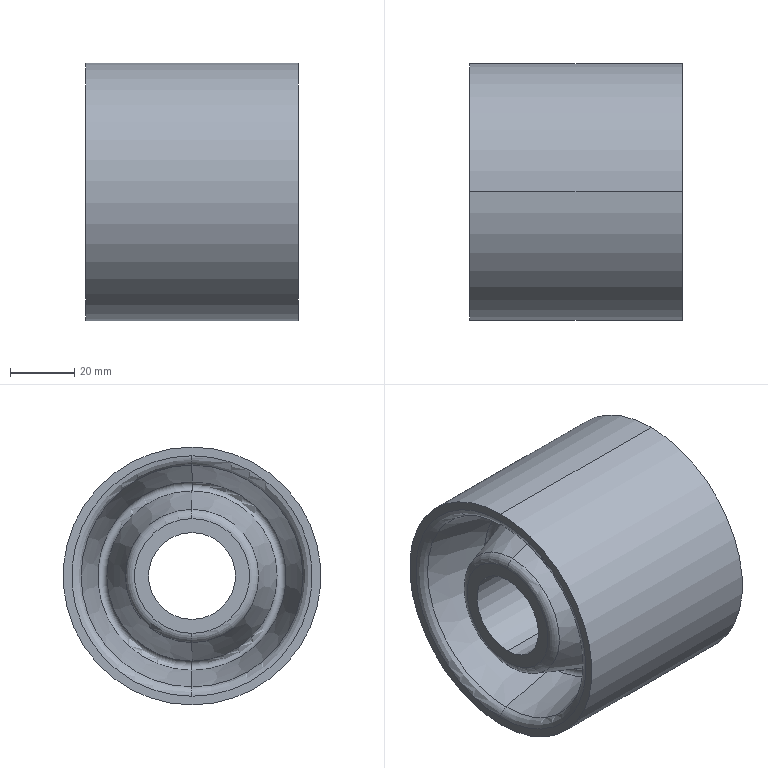Part | SolidWorks | features Revolution 1 | 1 solid | 28 faces | box 66 x 80 x 80 mm | volume 217017 mm3 | torus 12 | cone 8 | cylinder 4 | plane 4 | commonest cylinder face diameters 27 x2 80 x2
STEP:
#1=CARTESIAN_POINT('',(0.,0.,37.321));
#2=VERTEX_POINT('',#1);
#3=CARTESIAN_POINT('',(0.,0.,-37.321));
#4=VERTEX_POINT('',#3);
#5=CARTESIAN_POINT('',(0.,0.,0.));
#6=DIRECTION('',(-1.,0.,0.));
#7=DIRECTION('',(0.,0.,1.));
#8=AXIS2_PLACEMENT_3D('',#5,#6,#7);
#9=CIRCLE('',#8,37.321);
#10=EDGE_CURVE('',#2,#4,#9,.T.);
#11=ORIENTED_EDGE('',*,*,#10,.T.);
#12=CARTESIAN_POINT('',(2.247,0.,-34.417));
#13=VERTEX_POINT('',#12);
#14=CARTESIAN_POINT('',(3.,0.,-37.321));
#15=DIRECTION('',(0.,1.,0.));
#16=DIRECTION('',(0.,0.,1.));
#17=AXIS2_PLACEMENT_3D('',#14,#15,#16);
#18=CIRCLE('',#17,3.);
#19=EDGE_CURVE('',#4,#13,#18,.T.);
#20=ORIENTED_EDGE('',*,*,#19,.T.);
#21=CARTESIAN_POINT('',(2.247,0.,34.417));
#22=VERTEX_POINT('',#21);
#23=CARTESIAN_POINT('',(2.247,0.,0.));
#24=DIRECTION('',(-1.,0.,0.));
#25=DIRECTION('',(0.,0.,1.));
#26=AXIS2_PLACEMENT_3D('',#23,#24,#25);
#27=CIRCLE('',#26,34.417);
#28=EDGE_CURVE('',#22,#13,#27,.T.);
#29=ORIENTED_EDGE('',*,*,#28,.F.);
#30=CARTESIAN_POINT('',(3.,0.,37.321));
#31=DIRECTION('',(0.,-1.,0.));
#32=DIRECTION('',(0.,0.,-1.));
#33=AXIS2_PLACEMENT_3D('',#30,#31,#32);
#34=CIRCLE('',#33,3.);
#35=EDGE_CURVE('',#2,#22,#34,.T.);
#36=ORIENTED_EDGE('',*,*,#35,.F.);
#37=EDGE_LOOP('',(#11,#20,#29,#36));
#38=FACE_OUTER_BOUND('',#37,.T.);
#39=CARTESIAN_POINT('',(3.,0.,0.));
#40=DIRECTION('',(-1.,0.,0.));
#41=DIRECTION('',(0.,0.,1.));
#42=AXIS2_PLACEMENT_3D('',#39,#40,#41);
#43=TOROIDAL_SURFACE('',#42,37.321,3.);
#44=ADVANCED_FACE('',(#38),#43,.T.);
#45=CARTESIAN_POINT('',(22.093,0.,-29.272));
#46=VERTEX_POINT('',#45);
#47=CARTESIAN_POINT('',(22.093,0.,29.272));
#48=VERTEX_POINT('',#47);
#49=CARTESIAN_POINT('',(22.093,0.,0.));
#50=DIRECTION('',(-1.,0.,0.));
#51=DIRECTION('',(0.,0.,1.));
#52=AXIS2_PLACEMENT_3D('',#49,#50,#51);
#53=CIRCLE('',#52,29.272);
#54=EDGE_CURVE('',#46,#48,#53,.T.);
#55=ORIENTED_EDGE('',*,*,#54,.F.);
#56=CARTESIAN_POINT('',(2.247,0.,-34.417));
#57=DIRECTION('',(-0.968,0.,-0.251));
#58=VECTOR('',#57,1000.);
#59=LINE('',#56,#58);
#60=EDGE_CURVE('',#46,#13,#59,.T.);
#61=ORIENTED_EDGE('',*,*,#60,.T.);
#62=CARTESIAN_POINT('',(2.247,0.,0.));
#63=DIRECTION('',(-1.,0.,0.));
#64=DIRECTION('',(0.,0.,1.));
#65=AXIS2_PLACEMENT_3D('',#62,#63,#64);
#66=CIRCLE('',#65,34.417);
#67=EDGE_CURVE('',#13,#22,#66,.T.);
#68=ORIENTED_EDGE('',*,*,#67,.T.);
#69=CARTESIAN_POINT('',(2.247,0.,34.417));
#70=DIRECTION('',(-0.968,0.,0.251));
#71=VECTOR('',#70,1000.);
#72=LINE('',#69,#71);
#73=EDGE_CURVE('',#48,#22,#72,.T.);
#74=ORIENTED_EDGE('',*,*,#73,.F.);
#75=EDGE_LOOP('',(#55,#61,#68,#74));
#76=FACE_OUTER_BOUND('',#75,.T.);
#77=CARTESIAN_POINT('',(2.247,0.,0.));
#78=DIRECTION('',(-1.,0.,0.));
#79=DIRECTION('',(0.,0.,1.));
#80=AXIS2_PLACEMENT_3D('',#77,#78,#79);
#81=CONICAL_SURFACE('',#80,34.417,0.2537);
#82=ADVANCED_FACE('',(#76),#81,.F.);
#83=CARTESIAN_POINT('',(22.191,0.,-26.397));
#84=VERTEX_POINT('',#83);
#85=CARTESIAN_POINT('',(22.191,0.,26.397));
#86=VERTEX_POINT('',#85);
#87=CARTESIAN_POINT('',(22.191,0.,0.));
#88=DIRECTION('',(-1.,0.,0.));
#89=DIRECTION('',(0.,0.,1.));
#90=AXIS2_PLACEMENT_3D('',#87,#88,#89);
#91=CIRCLE('',#90,26.397);
#92=EDGE_CURVE('',#84,#86,#91,.T.);
#93=ORIENTED_EDGE('',*,*,#92,.F.);
#94=CARTESIAN_POINT('',(21.717,0.,-27.82));
#95=DIRECTION('',(0.,1.,0.));
#96=DIRECTION('',(0.,0.,1.));
#97=AXIS2_PLACEMENT_3D('',#94,#95,#96);
#98=CIRCLE('',#97,1.5);
#99=EDGE_CURVE('',#84,#46,#98,.T.);
#100=ORIENTED_EDGE('',*,*,#99,.T.);
#101=ORIENTED_EDGE('',*,*,#54,.T.);
#102=CARTESIAN_POINT('',(21.717,0.,27.82));
#103=DIRECTION('',(0.,-1.,0.));
#104=DIRECTION('',(0.,0.,-1.));
#105=AXIS2_PLACEMENT_3D('',#102,#103,#104);
#106=CIRCLE('',#105,1.5);
#107=EDGE_CURVE('',#86,#48,#106,.T.);
#108=ORIENTED_EDGE('',*,*,#107,.F.);
#109=EDGE_LOOP('',(#93,#100,#101,#108));
#110=FACE_OUTER_BOUND('',#109,.T.);
#111=CARTESIAN_POINT('',(21.717,0.,0.));
#112=DIRECTION('',(-1.,0.,0.));
#113=DIRECTION('',(0.,0.,1.));
#114=AXIS2_PLACEMENT_3D('',#111,#112,#113);
#115=TOROIDAL_SURFACE('',#114,27.82,1.5);
#116=ADVANCED_FACE('',(#110),#115,.F.);
#117=CARTESIAN_POINT('',(5.051,0.,20.684));
#118=VERTEX_POINT('',#117);
#119=CARTESIAN_POINT('',(5.051,0.,-20.684));
#120=VERTEX_POINT('',#119);
#121=CARTESIAN_POINT('',(5.051,0.,0.));
#122=DIRECTION('',(-1.,0.,0.));
#123=DIRECTION('',(0.,0.,1.));
#124=AXIS2_PLACEMENT_3D('',#121,#122,#123);
#125=CIRCLE('',#124,20.684);
#126=EDGE_CURVE('',#118,#120,#125,.T.);
#127=ORIENTED_EDGE('',*,*,#126,.F.);
#128=CARTESIAN_POINT('',(22.191,0.,26.397));
#129=DIRECTION('',(0.9487,0.,0.3162));
#130=VECTOR('',#129,1000.);
#131=LINE('',#128,#130);
#132=EDGE_CURVE('',#118,#86,#131,.T.);
#133=ORIENTED_EDGE('',*,*,#132,.T.);
#134=CARTESIAN_POINT('',(22.191,0.,0.));
#135=DIRECTION('',(-1.,0.,0.));
#136=DIRECTION('',(0.,0.,1.));
#137=AXIS2_PLACEMENT_3D('',#134,#135,#136);
#138=CIRCLE('',#137,26.397);
#139=EDGE_CURVE('',#86,#84,#138,.T.);
#140=ORIENTED_EDGE('',*,*,#139,.T.);
#141=CARTESIAN_POINT('',(22.191,0.,-26.397));
#142=DIRECTION('',(0.9487,0.,-0.3162));
#143=VECTOR('',#142,1000.);
#144=LINE('',#141,#143);
#145=EDGE_CURVE('',#120,#84,#144,.T.);
#146=ORIENTED_EDGE('',*,*,#145,.F.);
#147=EDGE_LOOP('',(#127,#133,#140,#146));
#148=FACE_OUTER_BOUND('',#147,.T.);
#149=CARTESIAN_POINT('',(22.191,0.,0.));
#150=DIRECTION('',(1.,0.,0.));
#151=DIRECTION('',(0.,0.,-1.));
#152=AXIS2_PLACEMENT_3D('',#149,#150,#151);
#153=CONICAL_SURFACE('',#152,26.397,0.3218);
#154=ADVANCED_FACE('',(#148),#153,.T.);
#155=ORIENTED_EDGE('',*,*,#126,.T.);
#156=CARTESIAN_POINT('',(3.,0.,-17.838));
#157=VERTEX_POINT('',#156);
#158=CARTESIAN_POINT('',(6.,0.,-17.838));
#159=DIRECTION('',(0.,1.,0.));
#160=DIRECTION('',(0.,0.,1.));
#161=AXIS2_PLACEMENT_3D('',#158,#159,#160);
#162=CIRCLE('',#161,3.);
#163=EDGE_CURVE('',#120,#157,#162,.T.);
#164=ORIENTED_EDGE('',*,*,#163,.T.);
#165=CARTESIAN_POINT('',(3.,0.,17.838));
#166=VERTEX_POINT('',#165);
#167=CARTESIAN_POINT('',(3.,0.,0.));
#168=DIRECTION('',(-1.,0.,0.));
#169=DIRECTION('',(0.,0.,1.));
#170=AXIS2_PLACEMENT_3D('',#167,#168,#169);
#171=CIRCLE('',#170,17.838);
#172=EDGE_CURVE('',#166,#157,#171,.T.);
#173=ORIENTED_EDGE('',*,*,#172,.F.);
#174=CARTESIAN_POINT('',(6.,0.,17.838));
#175=DIRECTION('',(0.,-1.,0.));
#176=DIRECTION('',(0.,0.,-1.));
#177=AXIS2_PLACEMENT_3D('',#174,#175,#176);
#178=CIRCLE('',#177,3.);
#179=EDGE_CURVE('',#118,#166,#178,.T.);
#180=ORIENTED_EDGE('',*,*,#179,.F.);
#181=EDGE_LOOP('',(#155,#164,#173,#180));
#182=FACE_OUTER_BOUND('',#181,.T.);
#183=CARTESIAN_POINT('',(6.,0.,0.));
#184=DIRECTION('',(-1.,0.,0.));
#185=DIRECTION('',(0.,0.,1.));
#186=AXIS2_PLACEMENT_3D('',#183,#184,#185);
#187=TOROIDAL_SURFACE('',#186,17.838,3.);
#188=ADVANCED_FACE('',(#182),#187,.T.);
#189=CARTESIAN_POINT('',(63.,0.,-13.5));
#190=VERTEX_POINT('',#189);
#191=CARTESIAN_POINT('',(63.,0.,13.5));
#192=VERTEX_POINT('',#191);
#193=CARTESIAN_POINT('',(63.,0.,0.));
#194=DIRECTION('',(-1.,0.,0.));
#195=DIRECTION('',(0.,0.,1.));
#196=AXIS2_PLACEMENT_3D('',#193,#194,#195);
#197=CIRCLE('',#196,13.5);
#198=EDGE_CURVE('',#190,#192,#197,.T.);
#199=ORIENTED_EDGE('',*,*,#198,.F.);
#200=CARTESIAN_POINT('',(3.,0.,-13.5));
#201=VERTEX_POINT('',#200);
#202=CARTESIAN_POINT('',(0.,0.,-13.5));
#203=DIRECTION('',(-1.,0.,0.));
#204=VECTOR('',#203,1000.);
#205=LINE('',#202,#204);
#206=EDGE_CURVE('',#190,#201,#205,.T.);
#207=ORIENTED_EDGE('',*,*,#206,.T.);
#208=CARTESIAN_POINT('',(3.,0.,13.5));
#209=VERTEX_POINT('',#208);
#210=CARTESIAN_POINT('',(3.,0.,0.));
#211=DIRECTION('',(-1.,0.,0.));
#212=DIRECTION('',(0.,0.,1.));
#213=AXIS2_PLACEMENT_3D('',#210,#211,#212);
#214=CIRCLE('',#213,13.5);
#215=EDGE_CURVE('',#201,#209,#214,.T.);
#216=ORIENTED_EDGE('',*,*,#215,.T.);
#217=CARTESIAN_POINT('',(0.,0.,13.5));
#218=DIRECTION('',(-1.,0.,0.));
#219=VECTOR('',#218,1000.);
#220=LINE('',#217,#219);
#221=EDGE_CURVE('',#192,#209,#220,.T.);
#222=ORIENTED_EDGE('',*,*,#221,.F.);
#223=EDGE_LOOP('',(#199,#207,#216,#222));
#224=FACE_OUTER_BOUND('',#223,.T.);
#225=CARTESIAN_POINT('',(0.,0.,0.));
#226=DIRECTION('',(-1.,0.,0.));
#227=DIRECTION('',(0.,0.,1.));
#228=AXIS2_PLACEMENT_3D('',#225,#226,#227);
#229=CYLINDRICAL_SURFACE('',#228,13.5);
#230=ADVANCED_FACE('',(#224),#229,.F.);
#231=CARTESIAN_POINT('',(63.,0.,17.838));
#232=VERTEX_POINT('',#231);
#233=CARTESIAN_POINT('',(63.,0.,-17.838));
#234=VERTEX_POINT('',#233);
#235=CARTESIAN_POINT('',(63.,0.,0.));
#236=DIRECTION('',(-1.,0.,0.));
#237=DIRECTION('',(0.,0.,1.));
#238=AXIS2_PLACEMENT_3D('',#235,#236,#237);
#239=CIRCLE('',#238,17.838);
#240=EDGE_CURVE('',#232,#234,#239,.T.);
#241=ORIENTED_EDGE('',*,*,#240,.T.);
#242=CARTESIAN_POINT('',(60.949,0.,-20.684));
#243=VERTEX_POINT('',#242);
#244=CARTESIAN_POINT('',(60.,0.,-17.838));
#245=DIRECTION('',(0.,1.,0.));
#246=DIRECTION('',(0.,0.,1.));
#247=AXIS2_PLACEMENT_3D('',#244,#245,#246);
#248=CIRCLE('',#247,3.);
#249=EDGE_CURVE('',#234,#243,#248,.T.);
#250=ORIENTED_EDGE('',*,*,#249,.T.);
#251=CARTESIAN_POINT('',(60.949,0.,20.684));
#252=VERTEX_POINT('',#251);
#253=CARTESIAN_POINT('',(60.949,0.,0.));
#254=DIRECTION('',(-1.,0.,0.));
#255=DIRECTION('',(0.,0.,1.));
#256=AXIS2_PLACEMENT_3D('',#253,#254,#255);
#257=CIRCLE('',#256,20.684);
#258=EDGE_CURVE('',#252,#243,#257,.T.);
#259=ORIENTED_EDGE('',*,*,#258,.F.);
#260=CARTESIAN_POINT('',(60.,0.,17.838));
#261=DIRECTION('',(0.,-1.,0.));
#262=DIRECTION('',(0.,0.,-1.));
#263=AXIS2_PLACEMENT_3D('',#260,#261,#262);
#264=CIRCLE('',#263,3.);
#265=EDGE_CURVE('',#232,#252,#264,.T.);
#266=ORIENTED_EDGE('',*,*,#265,.F.);
#267=EDGE_LOOP('',(#241,#250,#259,#266));
#268=FACE_OUTER_BOUND('',#267,.T.);
#269=CARTESIAN_POINT('',(60.,0.,0.));
#270=DIRECTION('',(-1.,0.,0.));
#271=DIRECTION('',(0.,0.,1.));
#272=AXIS2_PLACEMENT_3D('',#269,#270,#271);
#273=TOROIDAL_SURFACE('',#272,17.838,3.);
#274=ADVANCED_FACE('',(#268),#273,.T.);
#275=ORIENTED_EDGE('',*,*,#258,.T.);
#276=CARTESIAN_POINT('',(43.809,0.,-26.397));
#277=VERTEX_POINT('',#276);
#278=CARTESIAN_POINT('',(60.949,0.,-20.684));
#279=DIRECTION('',(-0.9487,0.,-0.3162));
#280=VECTOR('',#279,1000.);
#281=LINE('',#278,#280);
#282=EDGE_CURVE('',#243,#277,#281,.T.);
#283=ORIENTED_EDGE('',*,*,#282,.T.);
#284=CARTESIAN_POINT('',(43.809,0.,26.397));
#285=VERTEX_POINT('',#284);
#286=CARTESIAN_POINT('',(43.809,0.,0.));
#287=DIRECTION('',(-1.,0.,0.));
#288=DIRECTION('',(0.,0.,1.));
#289=AXIS2_PLACEMENT_3D('',#286,#287,#288);
#290=CIRCLE('',#289,26.397);
#291=EDGE_CURVE('',#285,#277,#290,.T.);
#292=ORIENTED_EDGE('',*,*,#291,.F.);
#293=CARTESIAN_POINT('',(60.949,0.,20.684));
#294=DIRECTION('',(-0.9487,0.,0.3162));
#295=VECTOR('',#294,1000.);
#296=LINE('',#293,#295);
#297=EDGE_CURVE('',#252,#285,#296,.T.);
#298=ORIENTED_EDGE('',*,*,#297,.F.);
#299=EDGE_LOOP('',(#275,#283,#292,#298));
#300=FACE_OUTER_BOUND('',#299,.T.);
#301=CARTESIAN_POINT('',(60.949,0.,0.));
#302=DIRECTION('',(-1.,0.,0.));
#303=DIRECTION('',(0.,0.,1.));
#304=AXIS2_PLACEMENT_3D('',#301,#302,#303);
#305=CONICAL_SURFACE('',#304,20.684,0.3218);
#306=ADVANCED_FACE('',(#300),#305,.T.);
#307=CARTESIAN_POINT('',(43.907,0.,-29.272));
#308=VERTEX_POINT('',#307);
#309=CARTESIAN_POINT('',(43.907,0.,29.272));
#310=VERTEX_POINT('',#309);
#311=CARTESIAN_POINT('',(43.907,0.,0.));
#312=DIRECTION('',(-1.,0.,0.));
#313=DIRECTION('',(0.,0.,1.));
#314=AXIS2_PLACEMENT_3D('',#311,#312,#313);
#315=CIRCLE('',#314,29.272);
#316=EDGE_CURVE('',#308,#310,#315,.T.);
#317=ORIENTED_EDGE('',*,*,#316,.F.);
#318=CARTESIAN_POINT('',(44.283,0.,-27.82));
#319=DIRECTION('',(0.,1.,0.));
#320=DIRECTION('',(0.,0.,1.));
#321=AXIS2_PLACEMENT_3D('',#318,#319,#320);
#322=CIRCLE('',#321,1.5);
#323=EDGE_CURVE('',#308,#277,#322,.T.);
#324=ORIENTED_EDGE('',*,*,#323,.T.);
#325=CARTESIAN_POINT('',(43.809,0.,0.));
#326=DIRECTION('',(-1.,0.,0.));
#327=DIRECTION('',(0.,0.,1.));
#328=AXIS2_PLACEMENT_3D('',#325,#326,#327);
#329=CIRCLE('',#328,26.397);
#330=EDGE_CURVE('',#277,#285,#329,.T.);
#331=ORIENTED_EDGE('',*,*,#330,.T.);
#332=CARTESIAN_POINT('',(44.283,0.,27.82));
#333=DIRECTION('',(0.,-1.,0.));
#334=DIRECTION('',(0.,0.,-1.));
#335=AXIS2_PLACEMENT_3D('',#332,#333,#334);
#336=CIRCLE('',#335,1.5);
#337=EDGE_CURVE('',#310,#285,#336,.T.);
#338=ORIENTED_EDGE('',*,*,#337,.F.);
#339=EDGE_LOOP('',(#317,#324,#331,#338));
#340=FACE_OUTER_BOUND('',#339,.T.);
#341=CARTESIAN_POINT('',(44.283,0.,0.));
#342=DIRECTION('',(-1.,0.,0.));
#343=DIRECTION('',(0.,0.,1.));
#344=AXIS2_PLACEMENT_3D('',#341,#342,#343);
#345=TOROIDAL_SURFACE('',#344,27.82,1.5);
#346=ADVANCED_FACE('',(#340),#345,.F.);
#347=ORIENTED_EDGE('',*,*,#316,.T.);
#348=CARTESIAN_POINT('',(63.753,0.,34.417));
#349=VERTEX_POINT('',#348);
#350=CARTESIAN_POINT('',(43.907,0.,29.272));
#351=DIRECTION('',(0.968,0.,0.251));
#352=VECTOR('',#351,1000.);
#353=LINE('',#350,#352);
#354=EDGE_CURVE('',#310,#349,#353,.T.);
#355=ORIENTED_EDGE('',*,*,#354,.T.);
#356=CARTESIAN_POINT('',(63.753,0.,-34.417));
#357=VERTEX_POINT('',#356);
#358=CARTESIAN_POINT('',(63.753,0.,0.));
#359=DIRECTION('',(-1.,0.,0.));
#360=DIRECTION('',(0.,0.,1.));
#361=AXIS2_PLACEMENT_3D('',#358,#359,#360);
#362=CIRCLE('',#361,34.417);
#363=EDGE_CURVE('',#357,#349,#362,.T.);
#364=ORIENTED_EDGE('',*,*,#363,.F.);
#365=CARTESIAN_POINT('',(43.907,0.,-29.272));
#366=DIRECTION('',(0.968,0.,-0.251));
#367=VECTOR('',#366,1000.);
#368=LINE('',#365,#367);
#369=EDGE_CURVE('',#308,#357,#368,.T.);
#370=ORIENTED_EDGE('',*,*,#369,.F.);
#371=EDGE_LOOP('',(#347,#355,#364,#370));
#372=FACE_OUTER_BOUND('',#371,.T.);
#373=CARTESIAN_POINT('',(43.907,0.,0.));
#374=DIRECTION('',(1.,0.,0.));
#375=DIRECTION('',(0.,0.,-1.));
#376=AXIS2_PLACEMENT_3D('',#373,#374,#375);
#377=CONICAL_SURFACE('',#376,29.272,0.2537);
#378=ADVANCED_FACE('',(#372),#377,.F.);
#379=CARTESIAN_POINT('',(63.753,0.,0.));
#380=DIRECTION('',(-1.,0.,0.));
#381=DIRECTION('',(0.,0.,1.));
#382=AXIS2_PLACEMENT_3D('',#379,#380,#381);
#383=CIRCLE('',#382,34.417);
#384=EDGE_CURVE('',#349,#357,#383,.T.);
#385=ORIENTED_EDGE('',*,*,#384,.T.);
#386=CARTESIAN_POINT('',(66.,0.,-37.321));
#387=VERTEX_POINT('',#386);
#388=CARTESIAN_POINT('',(63.,0.,-37.321));
#389=DIRECTION('',(0.,1.,0.));
#390=DIRECTION('',(0.,0.,1.));
#391=AXIS2_PLACEMENT_3D('',#388,#389,#390);
#392=CIRCLE('',#391,3.);
#393=EDGE_CURVE('',#357,#387,#392,.T.);
#394=ORIENTED_EDGE('',*,*,#393,.T.);
#395=CARTESIAN_POINT('',(66.,0.,37.321));
#396=VERTEX_POINT('',#395);
#397=CARTESIAN_POINT('',(66.,0.,0.));
#398=DIRECTION('',(-1.,0.,0.));
#399=DIRECTION('',(0.,0.,1.));
#400=AXIS2_PLACEMENT_3D('',#397,#398,#399);
#401=CIRCLE('',#400,37.321);
#402=EDGE_CURVE('',#396,#387,#401,.T.);
#403=ORIENTED_EDGE('',*,*,#402,.F.);
#404=CARTESIAN_POINT('',(63.,0.,37.321));
#405=DIRECTION('',(0.,-1.,0.));
#406=DIRECTION('',(0.,0.,-1.));
#407=AXIS2_PLACEMENT_3D('',#404,#405,#406);
#408=CIRCLE('',#407,3.);
#409=EDGE_CURVE('',#349,#396,#408,.T.);
#410=ORIENTED_EDGE('',*,*,#409,.F.);
#411=EDGE_LOOP('',(#385,#394,#403,#410));
#412=FACE_OUTER_BOUND('',#411,.T.);
#413=CARTESIAN_POINT('',(63.,0.,0.));
#414=DIRECTION('',(-1.,0.,0.));
#415=DIRECTION('',(0.,0.,1.));
#416=AXIS2_PLACEMENT_3D('',#413,#414,#415);
#417=TOROIDAL_SURFACE('',#416,37.321,3.);
#418=ADVANCED_FACE('',(#412),#417,.T.);
#419=CARTESIAN_POINT('',(66.,0.,40.));
#420=VERTEX_POINT('',#419);
#421=CARTESIAN_POINT('',(66.,0.,-40.));
#422=VERTEX_POINT('',#421);
#423=CARTESIAN_POINT('',(66.,0.,0.));
#424=DIRECTION('',(-1.,0.,0.));
#425=DIRECTION('',(0.,0.,1.));
#426=AXIS2_PLACEMENT_3D('',#423,#424,#425);
#427=CIRCLE('',#426,40.);
#428=EDGE_CURVE('',#420,#422,#427,.T.);
#429=ORIENTED_EDGE('',*,*,#428,.T.);
#430=CARTESIAN_POINT('',(0.,0.,-40.));
#431=VERTEX_POINT('',#430);
#432=CARTESIAN_POINT('',(0.,0.,-40.));
#433=DIRECTION('',(-1.,0.,0.));
#434=VECTOR('',#433,1000.);
#435=LINE('',#432,#434);
#436=EDGE_CURVE('',#422,#431,#435,.T.);
#437=ORIENTED_EDGE('',*,*,#436,.T.);
#438=CARTESIAN_POINT('',(0.,0.,40.));
#439=VERTEX_POINT('',#438);
#440=CARTESIAN_POINT('',(0.,0.,0.));
#441=DIRECTION('',(-1.,0.,0.));
#442=DIRECTION('',(0.,0.,1.));
#443=AXIS2_PLACEMENT_3D('',#440,#441,#442);
#444=CIRCLE('',#443,40.);
#445=EDGE_CURVE('',#439,#431,#444,.T.);
#446=ORIENTED_EDGE('',*,*,#445,.F.);
#447=CARTESIAN_POINT('',(0.,0.,40.));
#448=DIRECTION('',(-1.,0.,0.));
#449=VECTOR('',#448,1000.);
#450=LINE('',#447,#449);
#451=EDGE_CURVE('',#420,#439,#450,.T.);
#452=ORIENTED_EDGE('',*,*,#451,.F.);
#453=EDGE_LOOP('',(#429,#437,#446,#452));
#454=FACE_OUTER_BOUND('',#453,.T.);
#455=CARTESIAN_POINT('',(0.,0.,0.));
#456=DIRECTION('',(-1.,0.,0.));
#457=DIRECTION('',(0.,0.,1.));
#458=AXIS2_PLACEMENT_3D('',#455,#456,#457);
#459=CYLINDRICAL_SURFACE('',#458,40.);
#460=ADVANCED_FACE('',(#454),#459,.T.);
#461=ORIENTED_EDGE('',*,*,#10,.F.);
#462=CARTESIAN_POINT('',(0.,0.,0.));
#463=DIRECTION('',(-1.,0.,0.));
#464=DIRECTION('',(0.,0.,1.));
#465=AXIS2_PLACEMENT_3D('',#462,#463,#464);
#466=CIRCLE('',#465,37.321);
#467=EDGE_CURVE('',#4,#2,#466,.T.);
#468=ORIENTED_EDGE('',*,*,#467,.F.);
#469=EDGE_LOOP('',(#461,#468));
#470=FACE_BOUND('',#469,.T.);
#471=ORIENTED_EDGE('',*,*,#445,.T.);
#472=CARTESIAN_POINT('',(0.,0.,0.));
#473=DIRECTION('',(-1.,0.,0.));
#474=DIRECTION('',(0.,0.,1.));
#475=AXIS2_PLACEMENT_3D('',#472,#473,#474);
#476=CIRCLE('',#475,40.);
#477=EDGE_CURVE('',#431,#439,#476,.T.);
#478=ORIENTED_EDGE('',*,*,#477,.T.);
#479=EDGE_LOOP('',(#471,#478));
#480=FACE_OUTER_BOUND('',#479,.T.);
#481=CARTESIAN_POINT('',(0.,37.321,0.));
#482=DIRECTION('',(1.,0.,0.));
#483=DIRECTION('',(0.,0.,-1.));
#484=AXIS2_PLACEMENT_3D('',#481,#482,#483);
#485=PLANE('',#484);
#486=ADVANCED_FACE('',(#470,#480),#485,.F.);
#487=ORIENTED_EDGE('',*,*,#436,.F.);
#488=CARTESIAN_POINT('',(66.,0.,0.));
#489=DIRECTION('',(-1.,0.,0.));
#490=DIRECTION('',(0.,0.,1.));
#491=AXIS2_PLACEMENT_3D('',#488,#489,#490);
#492=CIRCLE('',#491,40.);
#493=EDGE_CURVE('',#422,#420,#492,.T.);
#494=ORIENTED_EDGE('',*,*,#493,.T.);
#495=ORIENTED_EDGE('',*,*,#451,.T.);
#496=ORIENTED_EDGE('',*,*,#477,.F.);
#497=EDGE_LOOP('',(#487,#494,#495,#496));
#498=FACE_OUTER_BOUND('',#497,.T.);
#499=CARTESIAN_POINT('',(0.,0.,0.));
#500=DIRECTION('',(-1.,0.,0.));
#501=DIRECTION('',(0.,0.,1.));
#502=AXIS2_PLACEMENT_3D('',#499,#500,#501);
#503=CYLINDRICAL_SURFACE('',#502,40.);
#504=ADVANCED_FACE('',(#498),#503,.T.);
#505=ORIENTED_EDGE('',*,*,#428,.F.);
#506=ORIENTED_EDGE('',*,*,#493,.F.);
#507=EDGE_LOOP('',(#505,#506));
#508=FACE_OUTER_BOUND('',#507,.T.);
#509=ORIENTED_EDGE('',*,*,#402,.T.);
#510=CARTESIAN_POINT('',(66.,0.,0.));
#511=DIRECTION('',(-1.,0.,0.));
#512=DIRECTION('',(0.,0.,1.));
#513=AXIS2_PLACEMENT_3D('',#510,#511,#512);
#514=CIRCLE('',#513,37.321);
#515=EDGE_CURVE('',#387,#396,#514,.T.);
#516=ORIENTED_EDGE('',*,*,#515,.T.);
#517=EDGE_LOOP('',(#509,#516));
#518=FACE_BOUND('',#517,.T.);
#519=CARTESIAN_POINT('',(66.,40.,0.));
#520=DIRECTION('',(-1.,0.,0.));
#521=DIRECTION('',(0.,0.,1.));
#522=AXIS2_PLACEMENT_3D('',#519,#520,#521);
#523=PLANE('',#522);
#524=ADVANCED_FACE('',(#508,#518),#523,.F.);
#525=ORIENTED_EDGE('',*,*,#393,.F.);
#526=ORIENTED_EDGE('',*,*,#363,.T.);
#527=ORIENTED_EDGE('',*,*,#409,.T.);
#528=ORIENTED_EDGE('',*,*,#515,.F.);
#529=EDGE_LOOP('',(#525,#526,#527,#528));
#530=FACE_OUTER_BOUND('',#529,.T.);
#531=CARTESIAN_POINT('',(63.,0.,0.));
#532=DIRECTION('',(-1.,0.,0.));
#533=DIRECTION('',(0.,0.,1.));
#534=AXIS2_PLACEMENT_3D('',#531,#532,#533);
#535=TOROIDAL_SURFACE('',#534,37.321,3.);
#536=ADVANCED_FACE('',(#530),#535,.T.);
#537=ORIENTED_EDGE('',*,*,#354,.F.);
#538=CARTESIAN_POINT('',(43.907,0.,0.));
#539=DIRECTION('',(-1.,0.,0.));
#540=DIRECTION('',(0.,0.,1.));
#541=AXIS2_PLACEMENT_3D('',#538,#539,#540);
#542=CIRCLE('',#541,29.272);
#543=EDGE_CURVE('',#310,#308,#542,.T.);
#544=ORIENTED_EDGE('',*,*,#543,.T.);
#545=ORIENTED_EDGE('',*,*,#369,.T.);
#546=ORIENTED_EDGE('',*,*,#384,.F.);
#547=EDGE_LOOP('',(#537,#544,#545,#546));
#548=FACE_OUTER_BOUND('',#547,.T.);
#549=CARTESIAN_POINT('',(43.907,0.,0.));
#550=DIRECTION('',(1.,0.,0.));
#551=DIRECTION('',(0.,0.,-1.));
#552=AXIS2_PLACEMENT_3D('',#549,#550,#551);
#553=CONICAL_SURFACE('',#552,29.272,0.2537);
#554=ADVANCED_FACE('',(#548),#553,.F.);
#555=ORIENTED_EDGE('',*,*,#323,.F.);
#556=ORIENTED_EDGE('',*,*,#543,.F.);
#557=ORIENTED_EDGE('',*,*,#337,.T.);
#558=ORIENTED_EDGE('',*,*,#291,.T.);
#559=EDGE_LOOP('',(#555,#556,#557,#558));
#560=FACE_OUTER_BOUND('',#559,.T.);
#561=CARTESIAN_POINT('',(44.283,0.,0.));
#562=DIRECTION('',(-1.,0.,0.));
#563=DIRECTION('',(0.,0.,1.));
#564=AXIS2_PLACEMENT_3D('',#561,#562,#563);
#565=TOROIDAL_SURFACE('',#564,27.82,1.5);
#566=ADVANCED_FACE('',(#560),#565,.F.);
#567=ORIENTED_EDGE('',*,*,#282,.F.);
#568=CARTESIAN_POINT('',(60.949,0.,0.));
#569=DIRECTION('',(-1.,0.,0.));
#570=DIRECTION('',(0.,0.,1.));
#571=AXIS2_PLACEMENT_3D('',#568,#569,#570);
#572=CIRCLE('',#571,20.684);
#573=EDGE_CURVE('',#243,#252,#572,.T.);
#574=ORIENTED_EDGE('',*,*,#573,.T.);
#575=ORIENTED_EDGE('',*,*,#297,.T.);
#576=ORIENTED_EDGE('',*,*,#330,.F.);
#577=EDGE_LOOP('',(#567,#574,#575,#576));
#578=FACE_OUTER_BOUND('',#577,.T.);
#579=CARTESIAN_POINT('',(60.949,0.,0.));
#580=DIRECTION('',(-1.,0.,0.));
#581=DIRECTION('',(0.,0.,1.));
#582=AXIS2_PLACEMENT_3D('',#579,#580,#581);
#583=CONICAL_SURFACE('',#582,20.684,0.3218);
#584=ADVANCED_FACE('',(#578),#583,.T.);
#585=ORIENTED_EDGE('',*,*,#249,.F.);
#586=CARTESIAN_POINT('',(63.,0.,0.));
#587=DIRECTION('',(-1.,0.,0.));
#588=DIRECTION('',(0.,0.,1.));
#589=AXIS2_PLACEMENT_3D('',#586,#587,#588);
#590=CIRCLE('',#589,17.838);
#591=EDGE_CURVE('',#234,#232,#590,.T.);
#592=ORIENTED_EDGE('',*,*,#591,.T.);
#593=ORIENTED_EDGE('',*,*,#265,.T.);
#594=ORIENTED_EDGE('',*,*,#573,.F.);
#595=EDGE_LOOP('',(#585,#592,#593,#594));
#596=FACE_OUTER_BOUND('',#595,.T.);
#597=CARTESIAN_POINT('',(60.,0.,0.));
#598=DIRECTION('',(-1.,0.,0.));
#599=DIRECTION('',(0.,0.,1.));
#600=AXIS2_PLACEMENT_3D('',#597,#598,#599);
#601=TOROIDAL_SURFACE('',#600,17.838,3.);
#602=ADVANCED_FACE('',(#596),#601,.T.);
#603=ORIENTED_EDGE('',*,*,#240,.F.);
#604=ORIENTED_EDGE('',*,*,#591,.F.);
#605=EDGE_LOOP('',(#603,#604));
#606=FACE_OUTER_BOUND('',#605,.T.);
#607=CARTESIAN_POINT('',(63.,0.,0.));
#608=DIRECTION('',(-1.,0.,0.));
#609=DIRECTION('',(0.,0.,1.));
#610=AXIS2_PLACEMENT_3D('',#607,#608,#609);
#611=CIRCLE('',#610,13.5);
#612=EDGE_CURVE('',#192,#190,#611,.T.);
#613=ORIENTED_EDGE('',*,*,#612,.T.);
#614=ORIENTED_EDGE('',*,*,#198,.T.);
#615=EDGE_LOOP('',(#613,#614));
#616=FACE_BOUND('',#615,.T.);
#617=CARTESIAN_POINT('',(63.,17.838,0.));
#618=DIRECTION('',(-1.,0.,0.));
#619=DIRECTION('',(0.,0.,1.));
#620=AXIS2_PLACEMENT_3D('',#617,#618,#619);
#621=PLANE('',#620);
#622=ADVANCED_FACE('',(#606,#616),#621,.F.);
#623=ORIENTED_EDGE('',*,*,#206,.F.);
#624=ORIENTED_EDGE('',*,*,#612,.F.);
#625=ORIENTED_EDGE('',*,*,#221,.T.);
#626=CARTESIAN_POINT('',(3.,0.,0.));
#627=DIRECTION('',(-1.,0.,0.));
#628=DIRECTION('',(0.,0.,1.));
#629=AXIS2_PLACEMENT_3D('',#626,#627,#628);
#630=CIRCLE('',#629,13.5);
#631=EDGE_CURVE('',#209,#201,#630,.T.);
#632=ORIENTED_EDGE('',*,*,#631,.T.);
#633=EDGE_LOOP('',(#623,#624,#625,#632));
#634=FACE_OUTER_BOUND('',#633,.T.);
#635=CARTESIAN_POINT('',(0.,0.,0.));
#636=DIRECTION('',(-1.,0.,0.));
#637=DIRECTION('',(0.,0.,1.));
#638=AXIS2_PLACEMENT_3D('',#635,#636,#637);
#639=CYLINDRICAL_SURFACE('',#638,13.5);
#640=ADVANCED_FACE('',(#634),#639,.F.);
#641=ORIENTED_EDGE('',*,*,#631,.F.);
#642=ORIENTED_EDGE('',*,*,#215,.F.);
#643=EDGE_LOOP('',(#641,#642));
#644=FACE_BOUND('',#643,.T.);
#645=ORIENTED_EDGE('',*,*,#172,.T.);
#646=CARTESIAN_POINT('',(3.,0.,0.));
#647=DIRECTION('',(-1.,0.,0.));
#648=DIRECTION('',(0.,0.,1.));
#649=AXIS2_PLACEMENT_3D('',#646,#647,#648);
#650=CIRCLE('',#649,17.838);
#651=EDGE_CURVE('',#157,#166,#650,.T.);
#652=ORIENTED_EDGE('',*,*,#651,.T.);
#653=EDGE_LOOP('',(#645,#652));
#654=FACE_OUTER_BOUND('',#653,.T.);
#655=CARTESIAN_POINT('',(3.,13.5,0.));
#656=DIRECTION('',(1.,0.,0.));
#657=DIRECTION('',(0.,0.,-1.));
#658=AXIS2_PLACEMENT_3D('',#655,#656,#657);
#659=PLANE('',#658);
#660=ADVANCED_FACE('',(#644,#654),#659,.F.);
#661=ORIENTED_EDGE('',*,*,#163,.F.);
#662=CARTESIAN_POINT('',(5.051,0.,0.));
#663=DIRECTION('',(-1.,0.,0.));
#664=DIRECTION('',(0.,0.,1.));
#665=AXIS2_PLACEMENT_3D('',#662,#663,#664);
#666=CIRCLE('',#665,20.684);
#667=EDGE_CURVE('',#120,#118,#666,.T.);
#668=ORIENTED_EDGE('',*,*,#667,.T.);
#669=ORIENTED_EDGE('',*,*,#179,.T.);
#670=ORIENTED_EDGE('',*,*,#651,.F.);
#671=EDGE_LOOP('',(#661,#668,#669,#670));
#672=FACE_OUTER_BOUND('',#671,.T.);
#673=CARTESIAN_POINT('',(6.,0.,0.));
#674=DIRECTION('',(-1.,0.,0.));
#675=DIRECTION('',(0.,0.,1.));
#676=AXIS2_PLACEMENT_3D('',#673,#674,#675);
#677=TOROIDAL_SURFACE('',#676,17.838,3.);
#678=ADVANCED_FACE('',(#672),#677,.T.);
#679=ORIENTED_EDGE('',*,*,#132,.F.);
#680=ORIENTED_EDGE('',*,*,#667,.F.);
#681=ORIENTED_EDGE('',*,*,#145,.T.);
#682=ORIENTED_EDGE('',*,*,#92,.T.);
#683=EDGE_LOOP('',(#679,#680,#681,#682));
#684=FACE_OUTER_BOUND('',#683,.T.);
#685=CARTESIAN_POINT('',(22.191,0.,0.));
#686=DIRECTION('',(1.,0.,0.));
#687=DIRECTION('',(0.,0.,-1.));
#688=AXIS2_PLACEMENT_3D('',#685,#686,#687);
#689=CONICAL_SURFACE('',#688,26.397,0.3218);
#690=ADVANCED_FACE('',(#684),#689,.T.);
#691=ORIENTED_EDGE('',*,*,#99,.F.);
#692=ORIENTED_EDGE('',*,*,#139,.F.);
#693=ORIENTED_EDGE('',*,*,#107,.T.);
#694=CARTESIAN_POINT('',(22.093,0.,0.));
#695=DIRECTION('',(-1.,0.,0.));
#696=DIRECTION('',(0.,0.,1.));
#697=AXIS2_PLACEMENT_3D('',#694,#695,#696);
#698=CIRCLE('',#697,29.272);
#699=EDGE_CURVE('',#48,#46,#698,.T.);
#700=ORIENTED_EDGE('',*,*,#699,.T.);
#701=EDGE_LOOP('',(#691,#692,#693,#700));
#702=FACE_OUTER_BOUND('',#701,.T.);
#703=CARTESIAN_POINT('',(21.717,0.,0.));
#704=DIRECTION('',(-1.,0.,0.));
#705=DIRECTION('',(0.,0.,1.));
#706=AXIS2_PLACEMENT_3D('',#703,#704,#705);
#707=TOROIDAL_SURFACE('',#706,27.82,1.5);
#708=ADVANCED_FACE('',(#702),#707,.F.);
#709=ORIENTED_EDGE('',*,*,#60,.F.);
#710=ORIENTED_EDGE('',*,*,#699,.F.);
#711=ORIENTED_EDGE('',*,*,#73,.T.);
#712=ORIENTED_EDGE('',*,*,#28,.T.);
#713=EDGE_LOOP('',(#709,#710,#711,#712));
#714=FACE_OUTER_BOUND('',#713,.T.);
#715=CARTESIAN_POINT('',(2.247,0.,0.));
#716=DIRECTION('',(-1.,0.,0.));
#717=DIRECTION('',(0.,0.,1.));
#718=AXIS2_PLACEMENT_3D('',#715,#716,#717);
#719=CONICAL_SURFACE('',#718,34.417,0.2537);
#720=ADVANCED_FACE('',(#714),#719,.F.);
#721=ORIENTED_EDGE('',*,*,#19,.F.);
#722=ORIENTED_EDGE('',*,*,#467,.T.);
#723=ORIENTED_EDGE('',*,*,#35,.T.);
#724=ORIENTED_EDGE('',*,*,#67,.F.);
#725=EDGE_LOOP('',(#721,#722,#723,#724));
#726=FACE_OUTER_BOUND('',#725,.T.);
#727=CARTESIAN_POINT('',(3.,0.,0.));
#728=DIRECTION('',(-1.,0.,0.));
#729=DIRECTION('',(0.,0.,1.));
#730=AXIS2_PLACEMENT_3D('',#727,#728,#729);
#731=TOROIDAL_SURFACE('',#730,37.321,3.);
#732=ADVANCED_FACE('',(#726),#731,.T.);
#733=CLOSED_SHELL('',(#44,#82,#116,#154,#188,#230,#274,#306,#346,#378,#418,#460,#486,#504,#524,#536,#554,#566,#584,#602,#622,#640,#660,#678,#690,#708,#720,#732));
#734=MANIFOLD_SOLID_BREP('',#733);
#735=CARTESIAN_POINT('',(0.,0.,0.));
#736=DIRECTION('',(0.,0.,1.));
#737=DIRECTION('',(1.,0.,0.));
#738=AXIS2_PLACEMENT_3D('',#735,#736,#737);
#739=(LENGTH_UNIT()NAMED_UNIT(*)SI_UNIT(.MILLI.,.METRE.));
#740=UNCERTAINTY_MEASURE_WITH_UNIT(LENGTH_MEASURE(0.00001),#739,'','');
#741=(NAMED_UNIT(*)PLANE_ANGLE_UNIT()SI_UNIT($,.RADIAN.));
#742=(NAMED_UNIT(*)SI_UNIT($,.STERADIAN.)SOLID_ANGLE_UNIT());
#743=(GEOMETRIC_REPRESENTATION_CONTEXT(3)GLOBAL_UNCERTAINTY_ASSIGNED_CONTEXT((#740))GLOBAL_UNIT_ASSIGNED_CONTEXT((#739,#741,#742))REPRESENTATION_CONTEXT('',''));
#744=ADVANCED_BREP_SHAPE_REPRESENTATION('',(#734,#738),#743);